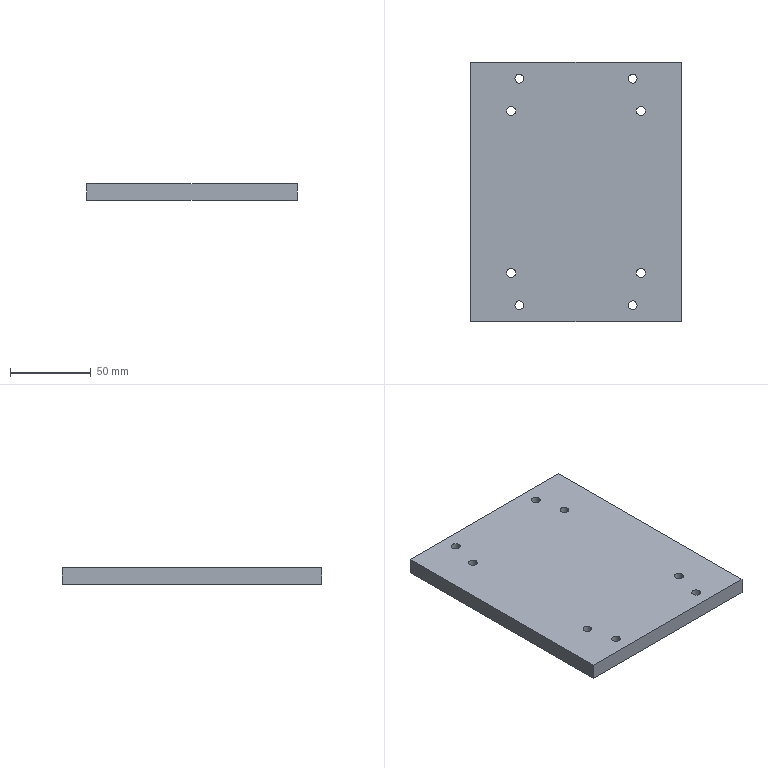Part | STEP file | B1-026 | 1 solid | 22 faces | box 130 x 160 x 10 mm | volume 206099 mm3 | cylinder 16 | plane 6 | commonest cylinder face diameters 5.5 x16